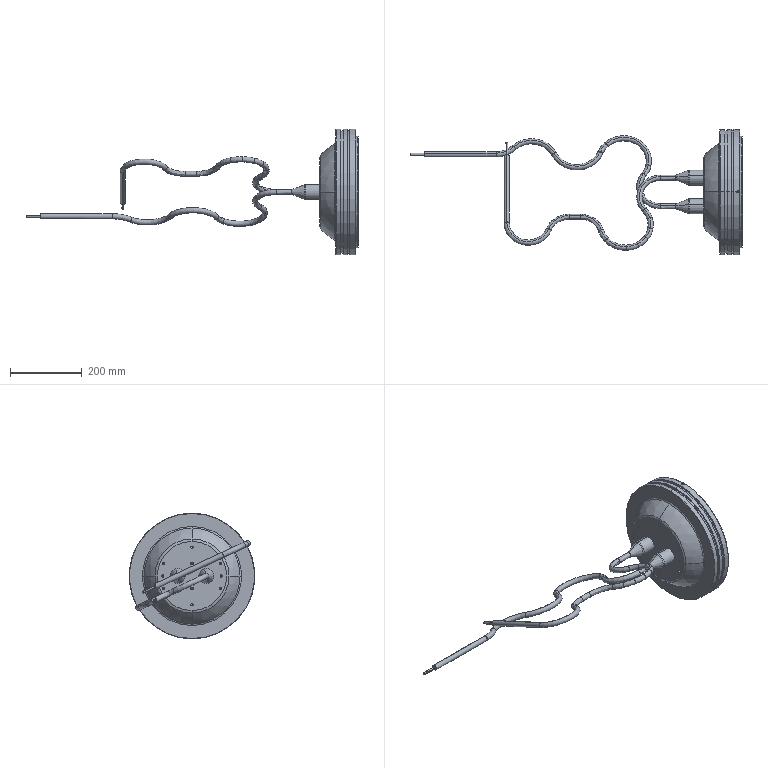Part | NX | features BREP 7 | 8 solids | 838 faces | box 924 x 350 x 350 mm | volume 7467445 mm3 | cylinder 285 | cone 195 | torus 135 | spline 119 | plane 100 | sphere 4 | commonest cylinder face diameters 30 x52 26 x48 1 x30 6.35 x29 14.5 x26 6.8 x18